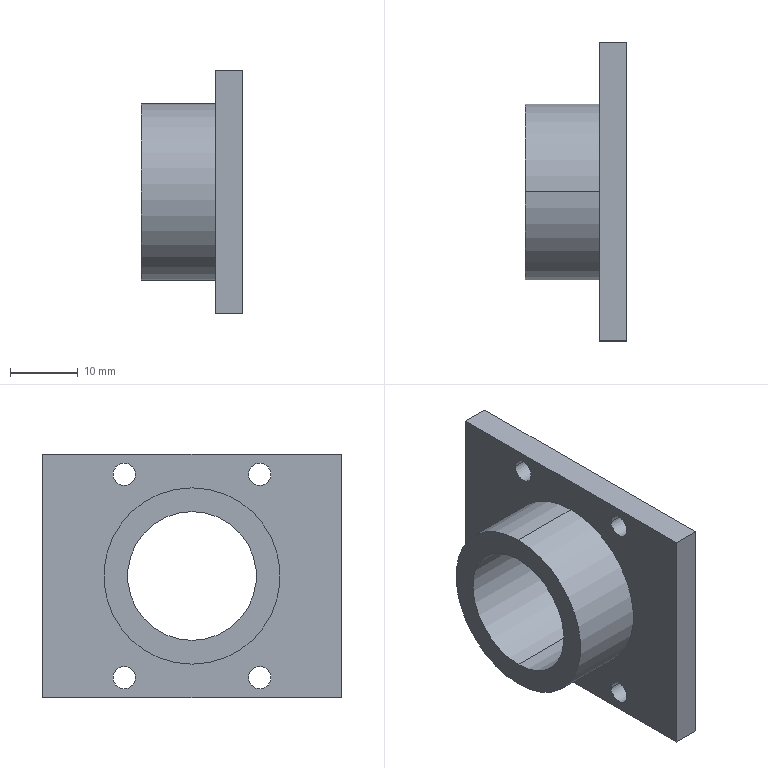Part | SolidWorks | features BaseBody 1 | 1 solid | 19 faces | box 15 x 44 x 36 mm | volume 7786 mm3 | cylinder 12 | plane 7 | commonest cylinder face diameters 3.3 x8 19 x2 26 x2
STEP:
#1=CARTESIAN_POINT('',(-2.,-11.65,33.));
#2=VERTEX_POINT('',#1);
#3=CARTESIAN_POINT('',(-2.,-8.35,33.));
#4=VERTEX_POINT('',#3);
#5=CARTESIAN_POINT('',(-2.,-10.,33.));
#6=DIRECTION('',(1.,0.,0.));
#7=DIRECTION('',(0.,1.,0.));
#8=AXIS2_PLACEMENT_3D('',#5,#6,#7);
#9=CIRCLE('',#8,1.65);
#10=EDGE_CURVE('',#2,#4,#9,.T.);
#11=ORIENTED_EDGE('',*,*,#10,.F.);
#12=CARTESIAN_POINT('',(2.,-11.65,33.));
#13=VERTEX_POINT('',#12);
#14=CARTESIAN_POINT('',(-14.2,-11.65,33.));
#15=DIRECTION('',(1.,0.,0.));
#16=VECTOR('',#15,1000.);
#17=LINE('',#14,#16);
#18=EDGE_CURVE('',#2,#13,#17,.T.);
#19=ORIENTED_EDGE('',*,*,#18,.T.);
#20=CARTESIAN_POINT('',(2.,-8.35,33.));
#21=VERTEX_POINT('',#20);
#22=CARTESIAN_POINT('',(2.,-10.,33.));
#23=DIRECTION('',(-1.,0.,0.));
#24=DIRECTION('',(0.,1.,0.));
#25=AXIS2_PLACEMENT_3D('',#22,#23,#24);
#26=CIRCLE('',#25,1.65);
#27=EDGE_CURVE('',#21,#13,#26,.T.);
#28=ORIENTED_EDGE('',*,*,#27,.F.);
#29=CARTESIAN_POINT('',(-14.2,-8.35,33.));
#30=DIRECTION('',(1.,0.,0.));
#31=VECTOR('',#30,1000.);
#32=LINE('',#29,#31);
#33=EDGE_CURVE('',#4,#21,#32,.T.);
#34=ORIENTED_EDGE('',*,*,#33,.F.);
#35=EDGE_LOOP('',(#11,#19,#28,#34));
#36=FACE_OUTER_BOUND('',#35,.T.);
#37=CARTESIAN_POINT('',(-14.2,-10.,33.));
#38=DIRECTION('',(1.,0.,0.));
#39=DIRECTION('',(0.,1.,0.));
#40=AXIS2_PLACEMENT_3D('',#37,#38,#39);
#41=CYLINDRICAL_SURFACE('',#40,1.65);
#42=ADVANCED_FACE('',(#36),#41,.F.);
#43=CARTESIAN_POINT('',(-13.,0.,27.5));
#44=VERTEX_POINT('',#43);
#45=CARTESIAN_POINT('',(-13.,0.,8.5));
#46=VERTEX_POINT('',#45);
#47=CARTESIAN_POINT('',(-13.,0.,18.));
#48=DIRECTION('',(1.,0.,0.));
#49=DIRECTION('',(0.,0.,-1.));
#50=AXIS2_PLACEMENT_3D('',#47,#48,#49);
#51=CIRCLE('',#50,9.5);
#52=EDGE_CURVE('',#44,#46,#51,.T.);
#53=ORIENTED_EDGE('',*,*,#52,.F.);
#54=CARTESIAN_POINT('',(2.,0.,27.5));
#55=VERTEX_POINT('',#54);
#56=CARTESIAN_POINT('',(-3.,0.,27.5));
#57=DIRECTION('',(1.,0.,0.));
#58=VECTOR('',#57,1000.);
#59=LINE('',#56,#58);
#60=EDGE_CURVE('',#44,#55,#59,.T.);
#61=ORIENTED_EDGE('',*,*,#60,.T.);
#62=CARTESIAN_POINT('',(2.,0.,8.5));
#63=VERTEX_POINT('',#62);
#64=CARTESIAN_POINT('',(2.,0.,18.));
#65=DIRECTION('',(-1.,0.,0.));
#66=DIRECTION('',(0.,0.,-1.));
#67=AXIS2_PLACEMENT_3D('',#64,#65,#66);
#68=CIRCLE('',#67,9.5);
#69=EDGE_CURVE('',#63,#55,#68,.T.);
#70=ORIENTED_EDGE('',*,*,#69,.F.);
#71=CARTESIAN_POINT('',(-3.,0.,8.5));
#72=DIRECTION('',(1.,0.,0.));
#73=VECTOR('',#72,1000.);
#74=LINE('',#71,#73);
#75=EDGE_CURVE('',#46,#63,#74,.T.);
#76=ORIENTED_EDGE('',*,*,#75,.F.);
#77=EDGE_LOOP('',(#53,#61,#70,#76));
#78=FACE_OUTER_BOUND('',#77,.T.);
#79=CARTESIAN_POINT('',(-3.,0.,18.));
#80=DIRECTION('',(1.,0.,0.));
#81=DIRECTION('',(0.,0.,-1.));
#82=AXIS2_PLACEMENT_3D('',#79,#80,#81);
#83=CYLINDRICAL_SURFACE('',#82,9.5);
#84=ADVANCED_FACE('',(#78),#83,.F.);
#85=CARTESIAN_POINT('',(-2.,-11.65,3.));
#86=VERTEX_POINT('',#85);
#87=CARTESIAN_POINT('',(-2.,-8.35,3.));
#88=VERTEX_POINT('',#87);
#89=CARTESIAN_POINT('',(-2.,-10.,3.));
#90=DIRECTION('',(1.,0.,0.));
#91=DIRECTION('',(0.,1.,0.));
#92=AXIS2_PLACEMENT_3D('',#89,#90,#91);
#93=CIRCLE('',#92,1.65);
#94=EDGE_CURVE('',#86,#88,#93,.T.);
#95=ORIENTED_EDGE('',*,*,#94,.F.);
#96=CARTESIAN_POINT('',(2.,-11.65,3.));
#97=VERTEX_POINT('',#96);
#98=CARTESIAN_POINT('',(-14.2,-11.65,3.));
#99=DIRECTION('',(1.,0.,0.));
#100=VECTOR('',#99,1000.);
#101=LINE('',#98,#100);
#102=EDGE_CURVE('',#86,#97,#101,.T.);
#103=ORIENTED_EDGE('',*,*,#102,.T.);
#104=CARTESIAN_POINT('',(2.,-8.35,3.));
#105=VERTEX_POINT('',#104);
#106=CARTESIAN_POINT('',(2.,-10.,3.));
#107=DIRECTION('',(-1.,0.,0.));
#108=DIRECTION('',(0.,1.,0.));
#109=AXIS2_PLACEMENT_3D('',#106,#107,#108);
#110=CIRCLE('',#109,1.65);
#111=EDGE_CURVE('',#105,#97,#110,.T.);
#112=ORIENTED_EDGE('',*,*,#111,.F.);
#113=CARTESIAN_POINT('',(-14.2,-8.35,3.));
#114=DIRECTION('',(1.,0.,0.));
#115=VECTOR('',#114,1000.);
#116=LINE('',#113,#115);
#117=EDGE_CURVE('',#88,#105,#116,.T.);
#118=ORIENTED_EDGE('',*,*,#117,.F.);
#119=EDGE_LOOP('',(#95,#103,#112,#118));
#120=FACE_OUTER_BOUND('',#119,.T.);
#121=CARTESIAN_POINT('',(-14.2,-10.,3.));
#122=DIRECTION('',(1.,0.,0.));
#123=DIRECTION('',(0.,1.,0.));
#124=AXIS2_PLACEMENT_3D('',#121,#122,#123);
#125=CYLINDRICAL_SURFACE('',#124,1.65);
#126=ADVANCED_FACE('',(#120),#125,.F.);
#127=CARTESIAN_POINT('',(-2.,8.35,33.));
#128=VERTEX_POINT('',#127);
#129=CARTESIAN_POINT('',(-2.,11.65,33.));
#130=VERTEX_POINT('',#129);
#131=CARTESIAN_POINT('',(-2.,10.,33.));
#132=DIRECTION('',(1.,0.,0.));
#133=DIRECTION('',(0.,1.,0.));
#134=AXIS2_PLACEMENT_3D('',#131,#132,#133);
#135=CIRCLE('',#134,1.65);
#136=EDGE_CURVE('',#128,#130,#135,.T.);
#137=ORIENTED_EDGE('',*,*,#136,.F.);
#138=CARTESIAN_POINT('',(2.,8.35,33.));
#139=VERTEX_POINT('',#138);
#140=CARTESIAN_POINT('',(-14.2,8.35,33.));
#141=DIRECTION('',(1.,0.,0.));
#142=VECTOR('',#141,1000.);
#143=LINE('',#140,#142);
#144=EDGE_CURVE('',#128,#139,#143,.T.);
#145=ORIENTED_EDGE('',*,*,#144,.T.);
#146=CARTESIAN_POINT('',(2.,11.65,33.));
#147=VERTEX_POINT('',#146);
#148=CARTESIAN_POINT('',(2.,10.,33.));
#149=DIRECTION('',(-1.,0.,0.));
#150=DIRECTION('',(0.,1.,0.));
#151=AXIS2_PLACEMENT_3D('',#148,#149,#150);
#152=CIRCLE('',#151,1.65);
#153=EDGE_CURVE('',#147,#139,#152,.T.);
#154=ORIENTED_EDGE('',*,*,#153,.F.);
#155=CARTESIAN_POINT('',(-14.2,11.65,33.));
#156=DIRECTION('',(1.,0.,0.));
#157=VECTOR('',#156,1000.);
#158=LINE('',#155,#157);
#159=EDGE_CURVE('',#130,#147,#158,.T.);
#160=ORIENTED_EDGE('',*,*,#159,.F.);
#161=EDGE_LOOP('',(#137,#145,#154,#160));
#162=FACE_OUTER_BOUND('',#161,.T.);
#163=CARTESIAN_POINT('',(-14.2,10.,33.));
#164=DIRECTION('',(1.,0.,0.));
#165=DIRECTION('',(0.,1.,0.));
#166=AXIS2_PLACEMENT_3D('',#163,#164,#165);
#167=CYLINDRICAL_SURFACE('',#166,1.65);
#168=ADVANCED_FACE('',(#162),#167,.F.);
#169=CARTESIAN_POINT('',(-2.,8.35,3.));
#170=VERTEX_POINT('',#169);
#171=CARTESIAN_POINT('',(-2.,11.65,3.));
#172=VERTEX_POINT('',#171);
#173=CARTESIAN_POINT('',(-2.,10.,3.));
#174=DIRECTION('',(1.,0.,0.));
#175=DIRECTION('',(0.,1.,0.));
#176=AXIS2_PLACEMENT_3D('',#173,#174,#175);
#177=CIRCLE('',#176,1.65);
#178=EDGE_CURVE('',#170,#172,#177,.T.);
#179=ORIENTED_EDGE('',*,*,#178,.F.);
#180=CARTESIAN_POINT('',(2.,8.35,3.));
#181=VERTEX_POINT('',#180);
#182=CARTESIAN_POINT('',(-14.2,8.35,3.));
#183=DIRECTION('',(1.,0.,0.));
#184=VECTOR('',#183,1000.);
#185=LINE('',#182,#184);
#186=EDGE_CURVE('',#170,#181,#185,.T.);
#187=ORIENTED_EDGE('',*,*,#186,.T.);
#188=CARTESIAN_POINT('',(2.,11.65,3.));
#189=VERTEX_POINT('',#188);
#190=CARTESIAN_POINT('',(2.,10.,3.));
#191=DIRECTION('',(-1.,0.,0.));
#192=DIRECTION('',(0.,1.,0.));
#193=AXIS2_PLACEMENT_3D('',#190,#191,#192);
#194=CIRCLE('',#193,1.65);
#195=EDGE_CURVE('',#189,#181,#194,.T.);
#196=ORIENTED_EDGE('',*,*,#195,.F.);
#197=CARTESIAN_POINT('',(-14.2,11.65,3.));
#198=DIRECTION('',(1.,0.,0.));
#199=VECTOR('',#198,1000.);
#200=LINE('',#197,#199);
#201=EDGE_CURVE('',#172,#189,#200,.T.);
#202=ORIENTED_EDGE('',*,*,#201,.F.);
#203=EDGE_LOOP('',(#179,#187,#196,#202));
#204=FACE_OUTER_BOUND('',#203,.T.);
#205=CARTESIAN_POINT('',(-14.2,10.,3.));
#206=DIRECTION('',(1.,0.,0.));
#207=DIRECTION('',(0.,1.,0.));
#208=AXIS2_PLACEMENT_3D('',#205,#206,#207);
#209=CYLINDRICAL_SURFACE('',#208,1.65);
#210=ADVANCED_FACE('',(#204),#209,.F.);
#211=CARTESIAN_POINT('',(-13.,0.,5.));
#212=VERTEX_POINT('',#211);
#213=CARTESIAN_POINT('',(-13.,0.,31.));
#214=VERTEX_POINT('',#213);
#215=CARTESIAN_POINT('',(-13.,0.,18.));
#216=DIRECTION('',(1.,0.,0.));
#217=DIRECTION('',(0.,0.,-1.));
#218=AXIS2_PLACEMENT_3D('',#215,#216,#217);
#219=CIRCLE('',#218,13.);
#220=EDGE_CURVE('',#212,#214,#219,.T.);
#221=ORIENTED_EDGE('',*,*,#220,.T.);
#222=CARTESIAN_POINT('',(-2.,0.,31.));
#223=VERTEX_POINT('',#222);
#224=CARTESIAN_POINT('',(-13.,0.,31.));
#225=DIRECTION('',(1.,0.,0.));
#226=VECTOR('',#225,1000.);
#227=LINE('',#224,#226);
#228=EDGE_CURVE('',#214,#223,#227,.T.);
#229=ORIENTED_EDGE('',*,*,#228,.T.);
#230=CARTESIAN_POINT('',(-2.,0.,5.));
#231=VERTEX_POINT('',#230);
#232=CARTESIAN_POINT('',(-2.,0.,18.));
#233=DIRECTION('',(-1.,0.,0.));
#234=DIRECTION('',(0.,0.,-1.));
#235=AXIS2_PLACEMENT_3D('',#232,#233,#234);
#236=CIRCLE('',#235,13.);
#237=EDGE_CURVE('',#223,#231,#236,.T.);
#238=ORIENTED_EDGE('',*,*,#237,.T.);
#239=CARTESIAN_POINT('',(-13.,0.,5.));
#240=DIRECTION('',(1.,0.,0.));
#241=VECTOR('',#240,1000.);
#242=LINE('',#239,#241);
#243=EDGE_CURVE('',#212,#231,#242,.T.);
#244=ORIENTED_EDGE('',*,*,#243,.F.);
#245=EDGE_LOOP('',(#221,#229,#238,#244));
#246=FACE_OUTER_BOUND('',#245,.T.);
#247=CARTESIAN_POINT('',(-13.,0.,18.));
#248=DIRECTION('',(1.,0.,0.));
#249=DIRECTION('',(0.,0.,-1.));
#250=AXIS2_PLACEMENT_3D('',#247,#248,#249);
#251=CYLINDRICAL_SURFACE('',#250,13.);
#252=ADVANCED_FACE('',(#246),#251,.T.);
#253=ORIENTED_EDGE('',*,*,#27,.T.);
#254=CARTESIAN_POINT('',(2.,-10.,33.));
#255=DIRECTION('',(-1.,0.,0.));
#256=DIRECTION('',(0.,1.,0.));
#257=AXIS2_PLACEMENT_3D('',#254,#255,#256);
#258=CIRCLE('',#257,1.65);
#259=EDGE_CURVE('',#13,#21,#258,.T.);
#260=ORIENTED_EDGE('',*,*,#259,.T.);
#261=EDGE_LOOP('',(#253,#260));
#262=FACE_BOUND('',#261,.T.);
#263=ORIENTED_EDGE('',*,*,#69,.T.);
#264=CARTESIAN_POINT('',(2.,0.,18.));
#265=DIRECTION('',(-1.,0.,0.));
#266=DIRECTION('',(0.,0.,-1.));
#267=AXIS2_PLACEMENT_3D('',#264,#265,#266);
#268=CIRCLE('',#267,9.5);
#269=EDGE_CURVE('',#55,#63,#268,.T.);
#270=ORIENTED_EDGE('',*,*,#269,.T.);
#271=EDGE_LOOP('',(#263,#270));
#272=FACE_BOUND('',#271,.T.);
#273=ORIENTED_EDGE('',*,*,#111,.T.);
#274=CARTESIAN_POINT('',(2.,-10.,3.));
#275=DIRECTION('',(-1.,0.,0.));
#276=DIRECTION('',(0.,1.,0.));
#277=AXIS2_PLACEMENT_3D('',#274,#275,#276);
#278=CIRCLE('',#277,1.65);
#279=EDGE_CURVE('',#97,#105,#278,.T.);
#280=ORIENTED_EDGE('',*,*,#279,.T.);
#281=EDGE_LOOP('',(#273,#280));
#282=FACE_BOUND('',#281,.T.);
#283=ORIENTED_EDGE('',*,*,#153,.T.);
#284=CARTESIAN_POINT('',(2.,10.,33.));
#285=DIRECTION('',(-1.,0.,0.));
#286=DIRECTION('',(0.,1.,0.));
#287=AXIS2_PLACEMENT_3D('',#284,#285,#286);
#288=CIRCLE('',#287,1.65);
#289=EDGE_CURVE('',#139,#147,#288,.T.);
#290=ORIENTED_EDGE('',*,*,#289,.T.);
#291=EDGE_LOOP('',(#283,#290));
#292=FACE_BOUND('',#291,.T.);
#293=ORIENTED_EDGE('',*,*,#195,.T.);
#294=CARTESIAN_POINT('',(2.,10.,3.));
#295=DIRECTION('',(-1.,0.,0.));
#296=DIRECTION('',(0.,1.,0.));
#297=AXIS2_PLACEMENT_3D('',#294,#295,#296);
#298=CIRCLE('',#297,1.65);
#299=EDGE_CURVE('',#181,#189,#298,.T.);
#300=ORIENTED_EDGE('',*,*,#299,.T.);
#301=EDGE_LOOP('',(#293,#300));
#302=FACE_BOUND('',#301,.T.);
#303=CARTESIAN_POINT('',(2.,22.,0.));
#304=VERTEX_POINT('',#303);
#305=CARTESIAN_POINT('',(2.,22.,36.));
#306=VERTEX_POINT('',#305);
#307=CARTESIAN_POINT('',(2.,22.,0.));
#308=DIRECTION('',(0.,0.,1.));
#309=VECTOR('',#308,1000.);
#310=LINE('',#307,#309);
#311=EDGE_CURVE('',#304,#306,#310,.T.);
#312=ORIENTED_EDGE('',*,*,#311,.T.);
#313=CARTESIAN_POINT('',(2.,-22.,36.));
#314=VERTEX_POINT('',#313);
#315=CARTESIAN_POINT('',(2.,-22.,36.));
#316=DIRECTION('',(0.,-1.,0.));
#317=VECTOR('',#316,1000.);
#318=LINE('',#315,#317);
#319=EDGE_CURVE('',#306,#314,#318,.T.);
#320=ORIENTED_EDGE('',*,*,#319,.T.);
#321=CARTESIAN_POINT('',(2.,-22.,0.));
#322=VERTEX_POINT('',#321);
#323=CARTESIAN_POINT('',(2.,-22.,0.));
#324=DIRECTION('',(0.,0.,-1.));
#325=VECTOR('',#324,1000.);
#326=LINE('',#323,#325);
#327=EDGE_CURVE('',#314,#322,#326,.T.);
#328=ORIENTED_EDGE('',*,*,#327,.T.);
#329=CARTESIAN_POINT('',(2.,-22.,0.));
#330=DIRECTION('',(0.,1.,0.));
#331=VECTOR('',#330,1000.);
#332=LINE('',#329,#331);
#333=EDGE_CURVE('',#322,#304,#332,.T.);
#334=ORIENTED_EDGE('',*,*,#333,.T.);
#335=EDGE_LOOP('',(#312,#320,#328,#334));
#336=FACE_OUTER_BOUND('',#335,.T.);
#337=CARTESIAN_POINT('',(2.,-22.,0.));
#338=DIRECTION('',(1.,0.,0.));
#339=DIRECTION('',(0.,0.,-1.));
#340=AXIS2_PLACEMENT_3D('',#337,#338,#339);
#341=PLANE('',#340);
#342=ADVANCED_FACE('',(#262,#272,#282,#292,#302,#336),#341,.T.);
#343=ORIENTED_EDGE('',*,*,#18,.F.);
#344=CARTESIAN_POINT('',(-2.,-10.,33.));
#345=DIRECTION('',(1.,0.,0.));
#346=DIRECTION('',(0.,1.,0.));
#347=AXIS2_PLACEMENT_3D('',#344,#345,#346);
#348=CIRCLE('',#347,1.65);
#349=EDGE_CURVE('',#4,#2,#348,.T.);
#350=ORIENTED_EDGE('',*,*,#349,.F.);
#351=ORIENTED_EDGE('',*,*,#33,.T.);
#352=ORIENTED_EDGE('',*,*,#259,.F.);
#353=EDGE_LOOP('',(#343,#350,#351,#352));
#354=FACE_OUTER_BOUND('',#353,.T.);
#355=CARTESIAN_POINT('',(-14.2,-10.,33.));
#356=DIRECTION('',(1.,0.,0.));
#357=DIRECTION('',(0.,1.,0.));
#358=AXIS2_PLACEMENT_3D('',#355,#356,#357);
#359=CYLINDRICAL_SURFACE('',#358,1.65);
#360=ADVANCED_FACE('',(#354),#359,.F.);
#361=ORIENTED_EDGE('',*,*,#60,.F.);
#362=CARTESIAN_POINT('',(-13.,0.,18.));
#363=DIRECTION('',(1.,0.,0.));
#364=DIRECTION('',(0.,0.,-1.));
#365=AXIS2_PLACEMENT_3D('',#362,#363,#364);
#366=CIRCLE('',#365,9.5);
#367=EDGE_CURVE('',#46,#44,#366,.T.);
#368=ORIENTED_EDGE('',*,*,#367,.F.);
#369=ORIENTED_EDGE('',*,*,#75,.T.);
#370=ORIENTED_EDGE('',*,*,#269,.F.);
#371=EDGE_LOOP('',(#361,#368,#369,#370));
#372=FACE_OUTER_BOUND('',#371,.T.);
#373=CARTESIAN_POINT('',(-3.,0.,18.));
#374=DIRECTION('',(1.,0.,0.));
#375=DIRECTION('',(0.,0.,-1.));
#376=AXIS2_PLACEMENT_3D('',#373,#374,#375);
#377=CYLINDRICAL_SURFACE('',#376,9.5);
#378=ADVANCED_FACE('',(#372),#377,.F.);
#379=ORIENTED_EDGE('',*,*,#102,.F.);
#380=CARTESIAN_POINT('',(-2.,-10.,3.));
#381=DIRECTION('',(1.,0.,0.));
#382=DIRECTION('',(0.,1.,0.));
#383=AXIS2_PLACEMENT_3D('',#380,#381,#382);
#384=CIRCLE('',#383,1.65);
#385=EDGE_CURVE('',#88,#86,#384,.T.);
#386=ORIENTED_EDGE('',*,*,#385,.F.);
#387=ORIENTED_EDGE('',*,*,#117,.T.);
#388=ORIENTED_EDGE('',*,*,#279,.F.);
#389=EDGE_LOOP('',(#379,#386,#387,#388));
#390=FACE_OUTER_BOUND('',#389,.T.);
#391=CARTESIAN_POINT('',(-14.2,-10.,3.));
#392=DIRECTION('',(1.,0.,0.));
#393=DIRECTION('',(0.,1.,0.));
#394=AXIS2_PLACEMENT_3D('',#391,#392,#393);
#395=CYLINDRICAL_SURFACE('',#394,1.65);
#396=ADVANCED_FACE('',(#390),#395,.F.);
#397=ORIENTED_EDGE('',*,*,#144,.F.);
#398=CARTESIAN_POINT('',(-2.,10.,33.));
#399=DIRECTION('',(1.,0.,0.));
#400=DIRECTION('',(0.,1.,0.));
#401=AXIS2_PLACEMENT_3D('',#398,#399,#400);
#402=CIRCLE('',#401,1.65);
#403=EDGE_CURVE('',#130,#128,#402,.T.);
#404=ORIENTED_EDGE('',*,*,#403,.F.);
#405=ORIENTED_EDGE('',*,*,#159,.T.);
#406=ORIENTED_EDGE('',*,*,#289,.F.);
#407=EDGE_LOOP('',(#397,#404,#405,#406));
#408=FACE_OUTER_BOUND('',#407,.T.);
#409=CARTESIAN_POINT('',(-14.2,10.,33.));
#410=DIRECTION('',(1.,0.,0.));
#411=DIRECTION('',(0.,1.,0.));
#412=AXIS2_PLACEMENT_3D('',#409,#410,#411);
#413=CYLINDRICAL_SURFACE('',#412,1.65);
#414=ADVANCED_FACE('',(#408),#413,.F.);
#415=ORIENTED_EDGE('',*,*,#186,.F.);
#416=CARTESIAN_POINT('',(-2.,10.,3.));
#417=DIRECTION('',(1.,0.,0.));
#418=DIRECTION('',(0.,1.,0.));
#419=AXIS2_PLACEMENT_3D('',#416,#417,#418);
#420=CIRCLE('',#419,1.65);
#421=EDGE_CURVE('',#172,#170,#420,.T.);
#422=ORIENTED_EDGE('',*,*,#421,.F.);
#423=ORIENTED_EDGE('',*,*,#201,.T.);
#424=ORIENTED_EDGE('',*,*,#299,.F.);
#425=EDGE_LOOP('',(#415,#422,#423,#424));
#426=FACE_OUTER_BOUND('',#425,.T.);
#427=CARTESIAN_POINT('',(-14.2,10.,3.));
#428=DIRECTION('',(1.,0.,0.));
#429=DIRECTION('',(0.,1.,0.));
#430=AXIS2_PLACEMENT_3D('',#427,#428,#429);
#431=CYLINDRICAL_SURFACE('',#430,1.65);
#432=ADVANCED_FACE('',(#426),#431,.F.);
#433=ORIENTED_EDGE('',*,*,#319,.F.);
#434=CARTESIAN_POINT('',(-2.,22.,36.));
#435=VERTEX_POINT('',#434);
#436=CARTESIAN_POINT('',(-2.,22.,36.));
#437=DIRECTION('',(-1.,0.,0.));
#438=VECTOR('',#437,1000.);
#439=LINE('',#436,#438);
#440=EDGE_CURVE('',#306,#435,#439,.T.);
#441=ORIENTED_EDGE('',*,*,#440,.T.);
#442=CARTESIAN_POINT('',(-2.,-22.,36.));
#443=VERTEX_POINT('',#442);
#444=CARTESIAN_POINT('',(-2.,-22.,36.));
#445=DIRECTION('',(0.,-1.,0.));
#446=VECTOR('',#445,1000.);
#447=LINE('',#444,#446);
#448=EDGE_CURVE('',#435,#443,#447,.T.);
#449=ORIENTED_EDGE('',*,*,#448,.T.);
#450=CARTESIAN_POINT('',(-2.,-22.,36.));
#451=DIRECTION('',(1.,0.,0.));
#452=VECTOR('',#451,1000.);
#453=LINE('',#450,#452);
#454=EDGE_CURVE('',#443,#314,#453,.T.);
#455=ORIENTED_EDGE('',*,*,#454,.T.);
#456=EDGE_LOOP('',(#433,#441,#449,#455));
#457=FACE_OUTER_BOUND('',#456,.T.);
#458=CARTESIAN_POINT('',(-2.,-22.,36.));
#459=DIRECTION('',(0.,0.,1.));
#460=DIRECTION('',(1.,0.,0.));
#461=AXIS2_PLACEMENT_3D('',#458,#459,#460);
#462=PLANE('',#461);
#463=ADVANCED_FACE('',(#457),#462,.T.);
#464=ORIENTED_EDGE('',*,*,#440,.F.);
#465=ORIENTED_EDGE('',*,*,#311,.F.);
#466=CARTESIAN_POINT('',(-2.,22.,0.));
#467=VERTEX_POINT('',#466);
#468=CARTESIAN_POINT('',(-2.,22.,0.));
#469=DIRECTION('',(-1.,0.,0.));
#470=VECTOR('',#469,1000.);
#471=LINE('',#468,#470);
#472=EDGE_CURVE('',#304,#467,#471,.T.);
#473=ORIENTED_EDGE('',*,*,#472,.T.);
#474=CARTESIAN_POINT('',(-2.,22.,0.));
#475=DIRECTION('',(0.,0.,1.));
#476=VECTOR('',#475,1000.);
#477=LINE('',#474,#476);
#478=EDGE_CURVE('',#467,#435,#477,.T.);
#479=ORIENTED_EDGE('',*,*,#478,.T.);
#480=EDGE_LOOP('',(#464,#465,#473,#479));
#481=FACE_OUTER_BOUND('',#480,.T.);
#482=CARTESIAN_POINT('',(-2.,22.,0.));
#483=DIRECTION('',(0.,1.,0.));
#484=DIRECTION('',(0.,0.,1.));
#485=AXIS2_PLACEMENT_3D('',#482,#483,#484);
#486=PLANE('',#485);
#487=ADVANCED_FACE('',(#481),#486,.T.);
#488=ORIENTED_EDGE('',*,*,#333,.F.);
#489=CARTESIAN_POINT('',(-2.,-22.,0.));
#490=VERTEX_POINT('',#489);
#491=CARTESIAN_POINT('',(-2.,-22.,0.));
#492=DIRECTION('',(1.,0.,0.));
#493=VECTOR('',#492,1000.);
#494=LINE('',#491,#493);
#495=EDGE_CURVE('',#490,#322,#494,.T.);
#496=ORIENTED_EDGE('',*,*,#495,.F.);
#497=CARTESIAN_POINT('',(-2.,-22.,0.));
#498=DIRECTION('',(0.,-1.,0.));
#499=VECTOR('',#498,1000.);
#500=LINE('',#497,#499);
#501=EDGE_CURVE('',#467,#490,#500,.T.);
#502=ORIENTED_EDGE('',*,*,#501,.F.);
#503=ORIENTED_EDGE('',*,*,#472,.F.);
#504=EDGE_LOOP('',(#488,#496,#502,#503));
#505=FACE_OUTER_BOUND('',#504,.T.);
#506=CARTESIAN_POINT('',(-2.,-22.,0.));
#507=DIRECTION('',(0.,0.,1.));
#508=DIRECTION('',(1.,0.,0.));
#509=AXIS2_PLACEMENT_3D('',#506,#507,#508);
#510=PLANE('',#509);
#511=ADVANCED_FACE('',(#505),#510,.F.);
#512=ORIENTED_EDGE('',*,*,#454,.F.);
#513=CARTESIAN_POINT('',(-2.,-22.,0.));
#514=DIRECTION('',(0.,0.,1.));
#515=VECTOR('',#514,1000.);
#516=LINE('',#513,#515);
#517=EDGE_CURVE('',#490,#443,#516,.T.);
#518=ORIENTED_EDGE('',*,*,#517,.F.);
#519=ORIENTED_EDGE('',*,*,#495,.T.);
#520=ORIENTED_EDGE('',*,*,#327,.F.);
#521=EDGE_LOOP('',(#512,#518,#519,#520));
#522=FACE_OUTER_BOUND('',#521,.T.);
#523=CARTESIAN_POINT('',(-2.,-22.,0.));
#524=DIRECTION('',(0.,1.,0.));
#525=DIRECTION('',(0.,0.,1.));
#526=AXIS2_PLACEMENT_3D('',#523,#524,#525);
#527=PLANE('',#526);
#528=ADVANCED_FACE('',(#522),#527,.F.);
#529=ORIENTED_EDGE('',*,*,#349,.T.);
#530=ORIENTED_EDGE('',*,*,#10,.T.);
#531=EDGE_LOOP('',(#529,#530));
#532=FACE_BOUND('',#531,.T.);
#533=CARTESIAN_POINT('',(-2.,0.,18.));
#534=DIRECTION('',(-1.,0.,0.));
#535=DIRECTION('',(0.,0.,-1.));
#536=AXIS2_PLACEMENT_3D('',#533,#534,#535);
#537=CIRCLE('',#536,13.);
#538=EDGE_CURVE('',#231,#223,#537,.T.);
#539=ORIENTED_EDGE('',*,*,#538,.F.);
#540=ORIENTED_EDGE('',*,*,#237,.F.);
#541=EDGE_LOOP('',(#539,#540));
#542=FACE_BOUND('',#541,.T.);
#543=ORIENTED_EDGE('',*,*,#385,.T.);
#544=ORIENTED_EDGE('',*,*,#94,.T.);
#545=EDGE_LOOP('',(#543,#544));
#546=FACE_BOUND('',#545,.T.);
#547=ORIENTED_EDGE('',*,*,#403,.T.);
#548=ORIENTED_EDGE('',*,*,#136,.T.);
#549=EDGE_LOOP('',(#547,#548));
#550=FACE_BOUND('',#549,.T.);
#551=ORIENTED_EDGE('',*,*,#421,.T.);
#552=ORIENTED_EDGE('',*,*,#178,.T.);
#553=EDGE_LOOP('',(#551,#552));
#554=FACE_BOUND('',#553,.T.);
#555=ORIENTED_EDGE('',*,*,#478,.F.);
#556=ORIENTED_EDGE('',*,*,#501,.T.);
#557=ORIENTED_EDGE('',*,*,#517,.T.);
#558=ORIENTED_EDGE('',*,*,#448,.F.);
#559=EDGE_LOOP('',(#555,#556,#557,#558));
#560=FACE_OUTER_BOUND('',#559,.T.);
#561=CARTESIAN_POINT('',(-2.,-22.,0.));
#562=DIRECTION('',(1.,0.,0.));
#563=DIRECTION('',(0.,0.,-1.));
#564=AXIS2_PLACEMENT_3D('',#561,#562,#563);
#565=PLANE('',#564);
#566=ADVANCED_FACE('',(#532,#542,#546,#550,#554,#560),#565,.F.);
#567=ORIENTED_EDGE('',*,*,#367,.T.);
#568=ORIENTED_EDGE('',*,*,#52,.T.);
#569=EDGE_LOOP('',(#567,#568));
#570=FACE_BOUND('',#569,.T.);
#571=ORIENTED_EDGE('',*,*,#220,.F.);
#572=CARTESIAN_POINT('',(-13.,0.,18.));
#573=DIRECTION('',(1.,0.,0.));
#574=DIRECTION('',(0.,0.,-1.));
#575=AXIS2_PLACEMENT_3D('',#572,#573,#574);
#576=CIRCLE('',#575,13.);
#577=EDGE_CURVE('',#214,#212,#576,.T.);
#578=ORIENTED_EDGE('',*,*,#577,.F.);
#579=EDGE_LOOP('',(#571,#578));
#580=FACE_OUTER_BOUND('',#579,.T.);
#581=CARTESIAN_POINT('',(-13.,0.,18.));
#582=DIRECTION('',(1.,0.,0.));
#583=DIRECTION('',(0.,0.,-1.));
#584=AXIS2_PLACEMENT_3D('',#581,#582,#583);
#585=PLANE('',#584);
#586=ADVANCED_FACE('',(#570,#580),#585,.F.);
#587=ORIENTED_EDGE('',*,*,#228,.F.);
#588=ORIENTED_EDGE('',*,*,#577,.T.);
#589=ORIENTED_EDGE('',*,*,#243,.T.);
#590=ORIENTED_EDGE('',*,*,#538,.T.);
#591=EDGE_LOOP('',(#587,#588,#589,#590));
#592=FACE_OUTER_BOUND('',#591,.T.);
#593=CARTESIAN_POINT('',(-13.,0.,18.));
#594=DIRECTION('',(1.,0.,0.));
#595=DIRECTION('',(0.,0.,-1.));
#596=AXIS2_PLACEMENT_3D('',#593,#594,#595);
#597=CYLINDRICAL_SURFACE('',#596,13.);
#598=ADVANCED_FACE('',(#592),#597,.T.);
#599=CLOSED_SHELL('',(#42,#84,#126,#168,#210,#252,#342,#360,#378,#396,#414,#432,#463,#487,#511,#528,#566,#586,#598));
#600=MANIFOLD_SOLID_BREP('',#599);
#601=CARTESIAN_POINT('',(0.,0.,0.));
#602=DIRECTION('',(0.,0.,1.));
#603=DIRECTION('',(1.,0.,0.));
#604=AXIS2_PLACEMENT_3D('',#601,#602,#603);
#605=(LENGTH_UNIT()NAMED_UNIT(*)SI_UNIT(.MILLI.,.METRE.));
#606=UNCERTAINTY_MEASURE_WITH_UNIT(LENGTH_MEASURE(0.00001),#605,'','');
#607=(NAMED_UNIT(*)PLANE_ANGLE_UNIT()SI_UNIT($,.RADIAN.));
#608=(NAMED_UNIT(*)SI_UNIT($,.STERADIAN.)SOLID_ANGLE_UNIT());
#609=(GEOMETRIC_REPRESENTATION_CONTEXT(3)GLOBAL_UNCERTAINTY_ASSIGNED_CONTEXT((#606))GLOBAL_UNIT_ASSIGNED_CONTEXT((#605,#607,#608))REPRESENTATION_CONTEXT('',''));
#610=ADVANCED_BREP_SHAPE_REPRESENTATION('',(#600,#604),#609);